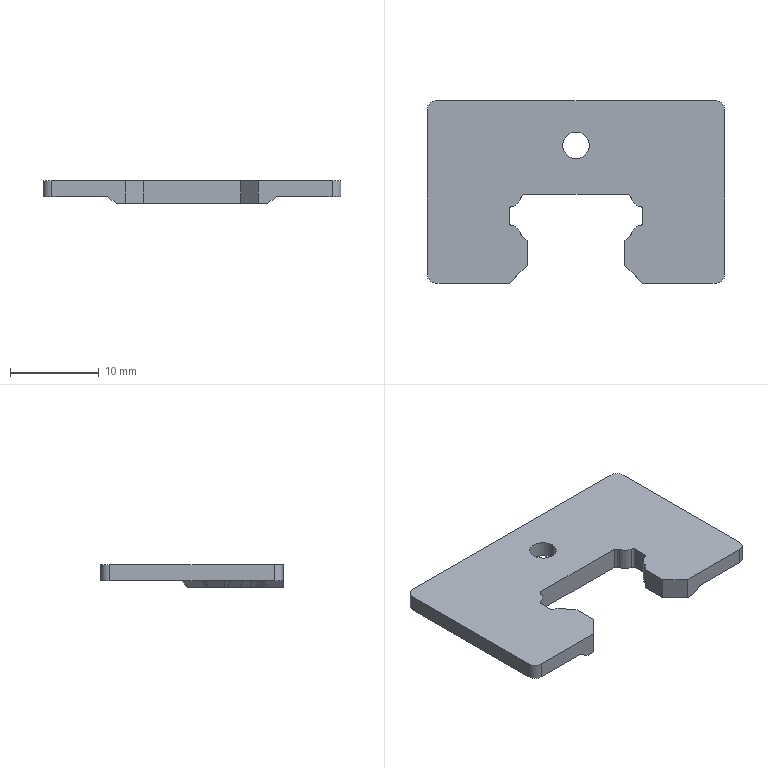Part | SolidWorks | features BaseBody 1 | 1 solid | 58 faces | box 33.5 x 20.5 x 2.5 mm | volume 1023 mm3 | plane 30 | cylinder 18 | cone 10 | commonest cylinder face diameters 0.6 x8 2 x4 2.6 x4 3 x2